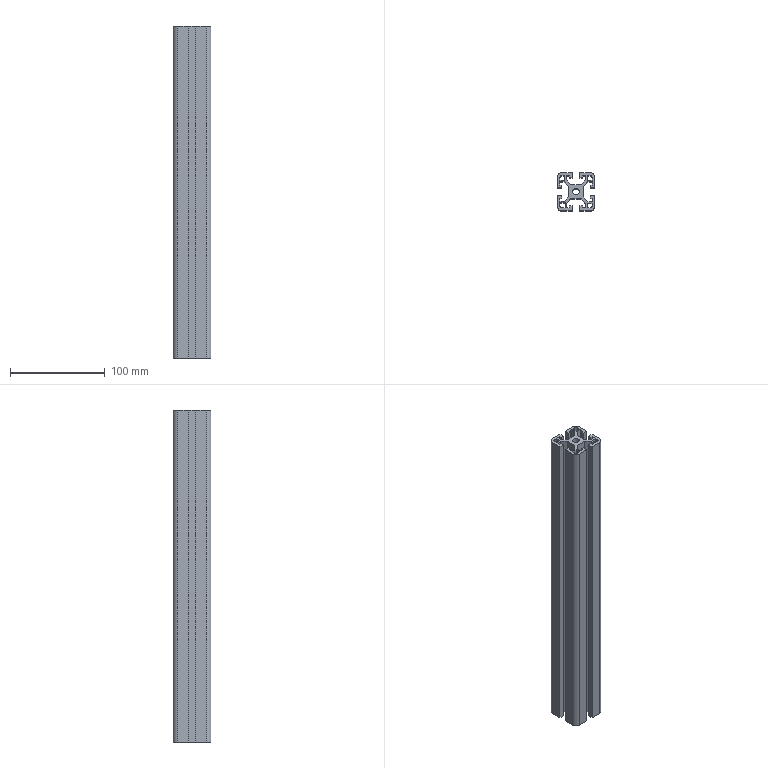Part | STEP file | 4040-350 | 1 solid | 88 faces | box 40 x 40 x 350 mm | volume 246381 mm3 | plane 78 | cylinder 10 | commonest cylinder face diameters 4 x4 10 x4 6.8 x2